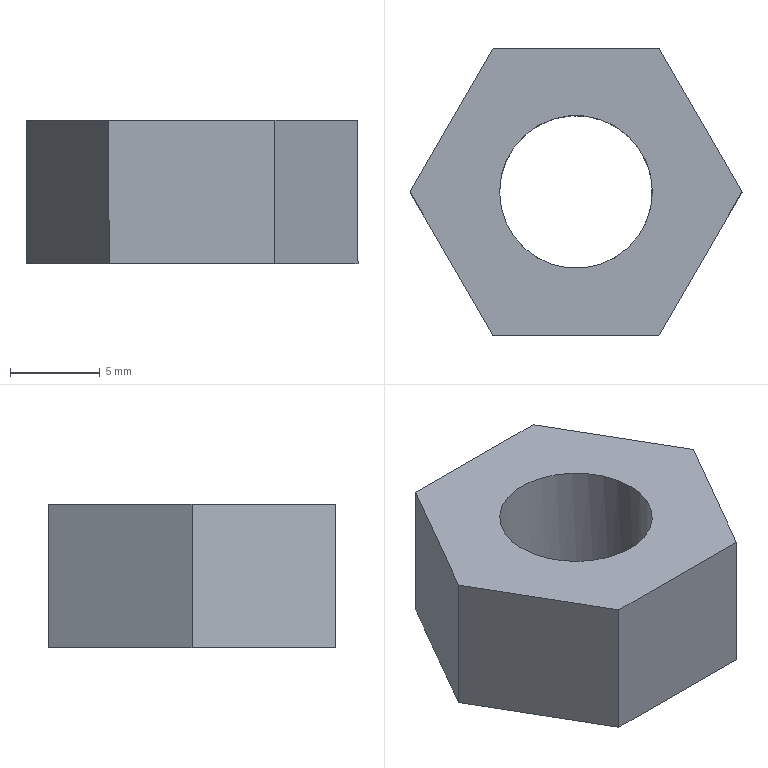Part | NX | 1 solid | 9 faces | box 18.475 x 16 x 8 mm | volume 1320 mm3 | plane 8 | cylinder 1 | commonest cylinder face diameters 8.5 x1
STEP:
#1=CARTESIAN_POINT('',(4.619,-8.,0.));
#2=VERTEX_POINT('',#1);
#3=CARTESIAN_POINT('',(9.238,0.,0.));
#4=VERTEX_POINT('',#3);
#5=CARTESIAN_POINT('',(4.619,-8.,0.));
#6=DIRECTION('',(0.5,0.866,0.));
#7=VECTOR('',#6,1000.);
#8=LINE('',#5,#7);
#9=EDGE_CURVE('',#2,#4,#8,.T.);
#10=ORIENTED_EDGE('',*,*,#9,.T.);
#11=CARTESIAN_POINT('',(9.238,0.,8.));
#12=VERTEX_POINT('',#11);
#13=CARTESIAN_POINT('',(9.238,0.,8.));
#14=DIRECTION('',(0.,0.,-1.));
#15=VECTOR('',#14,1000.);
#16=LINE('',#13,#15);
#17=EDGE_CURVE('',#12,#4,#16,.T.);
#18=ORIENTED_EDGE('',*,*,#17,.F.);
#19=CARTESIAN_POINT('',(4.619,-8.,8.));
#20=VERTEX_POINT('',#19);
#21=CARTESIAN_POINT('',(4.619,-8.,8.));
#22=DIRECTION('',(0.5,0.866,0.));
#23=VECTOR('',#22,1000.);
#24=LINE('',#21,#23);
#25=EDGE_CURVE('',#20,#12,#24,.T.);
#26=ORIENTED_EDGE('',*,*,#25,.F.);
#27=CARTESIAN_POINT('',(4.619,-8.,8.));
#28=DIRECTION('',(0.,0.,-1.));
#29=VECTOR('',#28,1000.);
#30=LINE('',#27,#29);
#31=EDGE_CURVE('',#20,#2,#30,.T.);
#32=ORIENTED_EDGE('',*,*,#31,.T.);
#33=EDGE_LOOP('',(#10,#18,#26,#32));
#34=FACE_BOUND('',#33,.T.);
#35=CARTESIAN_POINT('',(4.619,-8.,8.));
#36=DIRECTION('',(-0.866,0.5,0.));
#37=DIRECTION('',(-0.5,-0.866,0.));
#38=AXIS2_PLACEMENT_3D('',#35,#36,#37);
#39=PLANE('',#38);
#40=ADVANCED_FACE('',(#34),#39,.F.);
#41=CARTESIAN_POINT('',(4.619,8.,0.));
#42=VERTEX_POINT('',#41);
#43=CARTESIAN_POINT('',(9.238,0.,0.));
#44=DIRECTION('',(-0.5,0.866,0.));
#45=VECTOR('',#44,1000.);
#46=LINE('',#43,#45);
#47=EDGE_CURVE('',#4,#42,#46,.T.);
#48=ORIENTED_EDGE('',*,*,#47,.T.);
#49=CARTESIAN_POINT('',(4.619,8.,8.));
#50=VERTEX_POINT('',#49);
#51=CARTESIAN_POINT('',(4.619,8.,8.));
#52=DIRECTION('',(0.,0.,-1.));
#53=VECTOR('',#52,1000.);
#54=LINE('',#51,#53);
#55=EDGE_CURVE('',#50,#42,#54,.T.);
#56=ORIENTED_EDGE('',*,*,#55,.F.);
#57=CARTESIAN_POINT('',(9.238,0.,8.));
#58=DIRECTION('',(-0.5,0.866,0.));
#59=VECTOR('',#58,1000.);
#60=LINE('',#57,#59);
#61=EDGE_CURVE('',#12,#50,#60,.T.);
#62=ORIENTED_EDGE('',*,*,#61,.F.);
#63=ORIENTED_EDGE('',*,*,#17,.T.);
#64=EDGE_LOOP('',(#48,#56,#62,#63));
#65=FACE_BOUND('',#64,.T.);
#66=CARTESIAN_POINT('',(9.238,0.,8.));
#67=DIRECTION('',(-0.866,-0.5,0.));
#68=DIRECTION('',(0.5,-0.866,0.));
#69=AXIS2_PLACEMENT_3D('',#66,#67,#68);
#70=PLANE('',#69);
#71=ADVANCED_FACE('',(#65),#70,.F.);
#72=CARTESIAN_POINT('',(-4.619,8.,0.));
#73=VERTEX_POINT('',#72);
#74=CARTESIAN_POINT('',(4.619,8.,0.));
#75=DIRECTION('',(-1.,0.,0.));
#76=VECTOR('',#75,1000.);
#77=LINE('',#74,#76);
#78=EDGE_CURVE('',#42,#73,#77,.T.);
#79=ORIENTED_EDGE('',*,*,#78,.T.);
#80=CARTESIAN_POINT('',(-4.619,8.,8.));
#81=VERTEX_POINT('',#80);
#82=CARTESIAN_POINT('',(-4.619,8.,8.));
#83=DIRECTION('',(0.,0.,-1.));
#84=VECTOR('',#83,1000.);
#85=LINE('',#82,#84);
#86=EDGE_CURVE('',#81,#73,#85,.T.);
#87=ORIENTED_EDGE('',*,*,#86,.F.);
#88=CARTESIAN_POINT('',(4.619,8.,8.));
#89=DIRECTION('',(-1.,0.,0.));
#90=VECTOR('',#89,1000.);
#91=LINE('',#88,#90);
#92=EDGE_CURVE('',#50,#81,#91,.T.);
#93=ORIENTED_EDGE('',*,*,#92,.F.);
#94=ORIENTED_EDGE('',*,*,#55,.T.);
#95=EDGE_LOOP('',(#79,#87,#93,#94));
#96=FACE_BOUND('',#95,.T.);
#97=CARTESIAN_POINT('',(4.619,8.,8.));
#98=DIRECTION('',(0.,-1.,0.));
#99=DIRECTION('',(0.,0.,-1.));
#100=AXIS2_PLACEMENT_3D('',#97,#98,#99);
#101=PLANE('',#100);
#102=ADVANCED_FACE('',(#96),#101,.F.);
#103=CARTESIAN_POINT('',(-9.238,0.,0.));
#104=VERTEX_POINT('',#103);
#105=CARTESIAN_POINT('',(-4.619,8.,0.));
#106=DIRECTION('',(-0.5,-0.866,0.));
#107=VECTOR('',#106,1000.);
#108=LINE('',#105,#107);
#109=EDGE_CURVE('',#73,#104,#108,.T.);
#110=ORIENTED_EDGE('',*,*,#109,.T.);
#111=CARTESIAN_POINT('',(-9.238,0.,8.));
#112=VERTEX_POINT('',#111);
#113=CARTESIAN_POINT('',(-9.238,0.,8.));
#114=DIRECTION('',(0.,0.,-1.));
#115=VECTOR('',#114,1000.);
#116=LINE('',#113,#115);
#117=EDGE_CURVE('',#112,#104,#116,.T.);
#118=ORIENTED_EDGE('',*,*,#117,.F.);
#119=CARTESIAN_POINT('',(-4.619,8.,8.));
#120=DIRECTION('',(-0.5,-0.866,0.));
#121=VECTOR('',#120,1000.);
#122=LINE('',#119,#121);
#123=EDGE_CURVE('',#81,#112,#122,.T.);
#124=ORIENTED_EDGE('',*,*,#123,.F.);
#125=ORIENTED_EDGE('',*,*,#86,.T.);
#126=EDGE_LOOP('',(#110,#118,#124,#125));
#127=FACE_BOUND('',#126,.T.);
#128=CARTESIAN_POINT('',(-4.619,8.,8.));
#129=DIRECTION('',(0.866,-0.5,0.));
#130=DIRECTION('',(0.5,0.866,0.));
#131=AXIS2_PLACEMENT_3D('',#128,#129,#130);
#132=PLANE('',#131);
#133=ADVANCED_FACE('',(#127),#132,.F.);
#134=CARTESIAN_POINT('',(-4.619,-8.,0.));
#135=VERTEX_POINT('',#134);
#136=CARTESIAN_POINT('',(-9.238,0.,0.));
#137=DIRECTION('',(0.5,-0.866,0.));
#138=VECTOR('',#137,1000.);
#139=LINE('',#136,#138);
#140=EDGE_CURVE('',#104,#135,#139,.T.);
#141=ORIENTED_EDGE('',*,*,#140,.T.);
#142=CARTESIAN_POINT('',(-4.619,-8.,8.));
#143=VERTEX_POINT('',#142);
#144=CARTESIAN_POINT('',(-4.619,-8.,8.));
#145=DIRECTION('',(0.,0.,-1.));
#146=VECTOR('',#145,1000.);
#147=LINE('',#144,#146);
#148=EDGE_CURVE('',#143,#135,#147,.T.);
#149=ORIENTED_EDGE('',*,*,#148,.F.);
#150=CARTESIAN_POINT('',(-9.238,0.,8.));
#151=DIRECTION('',(0.5,-0.866,0.));
#152=VECTOR('',#151,1000.);
#153=LINE('',#150,#152);
#154=EDGE_CURVE('',#112,#143,#153,.T.);
#155=ORIENTED_EDGE('',*,*,#154,.F.);
#156=ORIENTED_EDGE('',*,*,#117,.T.);
#157=EDGE_LOOP('',(#141,#149,#155,#156));
#158=FACE_BOUND('',#157,.T.);
#159=CARTESIAN_POINT('',(-9.238,0.,8.));
#160=DIRECTION('',(0.866,0.5,0.));
#161=DIRECTION('',(-0.5,0.866,0.));
#162=AXIS2_PLACEMENT_3D('',#159,#160,#161);
#163=PLANE('',#162);
#164=ADVANCED_FACE('',(#158),#163,.F.);
#165=CARTESIAN_POINT('',(-4.619,-8.,0.));
#166=DIRECTION('',(1.,0.,0.));
#167=VECTOR('',#166,1000.);
#168=LINE('',#165,#167);
#169=EDGE_CURVE('',#135,#2,#168,.T.);
#170=ORIENTED_EDGE('',*,*,#169,.T.);
#171=ORIENTED_EDGE('',*,*,#31,.F.);
#172=CARTESIAN_POINT('',(-4.619,-8.,8.));
#173=DIRECTION('',(1.,0.,0.));
#174=VECTOR('',#173,1000.);
#175=LINE('',#172,#174);
#176=EDGE_CURVE('',#143,#20,#175,.T.);
#177=ORIENTED_EDGE('',*,*,#176,.F.);
#178=ORIENTED_EDGE('',*,*,#148,.T.);
#179=EDGE_LOOP('',(#170,#171,#177,#178));
#180=FACE_BOUND('',#179,.T.);
#181=CARTESIAN_POINT('',(-4.619,-8.,8.));
#182=DIRECTION('',(0.,1.,0.));
#183=DIRECTION('',(-1.,0.,0.));
#184=AXIS2_PLACEMENT_3D('',#181,#182,#183);
#185=PLANE('',#184);
#186=ADVANCED_FACE('',(#180),#185,.F.);
#187=CARTESIAN_POINT('',(4.25,0.,8.));
#188=VERTEX_POINT('',#187);
#189=CARTESIAN_POINT('',(0.,0.,8.));
#190=DIRECTION('',(0.,0.,1.));
#191=DIRECTION('',(1.,0.,0.));
#192=AXIS2_PLACEMENT_3D('',#189,#190,#191);
#193=CIRCLE('',#192,4.25);
#194=EDGE_CURVE('',#188,#188,#193,.T.);
#195=ORIENTED_EDGE('',*,*,#194,.F.);
#196=EDGE_LOOP('',(#195));
#197=FACE_BOUND('',#196,.T.);
#198=ORIENTED_EDGE('',*,*,#25,.T.);
#199=ORIENTED_EDGE('',*,*,#61,.T.);
#200=ORIENTED_EDGE('',*,*,#92,.T.);
#201=ORIENTED_EDGE('',*,*,#123,.T.);
#202=ORIENTED_EDGE('',*,*,#154,.T.);
#203=ORIENTED_EDGE('',*,*,#176,.T.);
#204=EDGE_LOOP('',(#198,#199,#200,#201,#202,#203));
#205=FACE_BOUND('',#204,.T.);
#206=CARTESIAN_POINT('',(0.,0.,8.));
#207=DIRECTION('',(0.,0.,1.));
#208=DIRECTION('',(1.,0.,0.));
#209=AXIS2_PLACEMENT_3D('',#206,#207,#208);
#210=PLANE('',#209);
#211=ADVANCED_FACE('',(#197,#205),#210,.T.);
#212=CARTESIAN_POINT('',(-4.25,0.,0.));
#213=VERTEX_POINT('',#212);
#214=CARTESIAN_POINT('',(0.,0.,0.));
#215=DIRECTION('',(0.,0.,-1.));
#216=DIRECTION('',(-1.,0.,0.));
#217=AXIS2_PLACEMENT_3D('',#214,#215,#216);
#218=CIRCLE('',#217,4.25);
#219=EDGE_CURVE('',#213,#213,#218,.T.);
#220=ORIENTED_EDGE('',*,*,#219,.F.);
#221=EDGE_LOOP('',(#220));
#222=FACE_BOUND('',#221,.T.);
#223=ORIENTED_EDGE('',*,*,#9,.F.);
#224=ORIENTED_EDGE('',*,*,#169,.F.);
#225=ORIENTED_EDGE('',*,*,#140,.F.);
#226=ORIENTED_EDGE('',*,*,#109,.F.);
#227=ORIENTED_EDGE('',*,*,#78,.F.);
#228=ORIENTED_EDGE('',*,*,#47,.F.);
#229=EDGE_LOOP('',(#223,#224,#225,#226,#227,#228));
#230=FACE_BOUND('',#229,.T.);
#231=CARTESIAN_POINT('',(0.,0.,0.));
#232=DIRECTION('',(0.,0.,1.));
#233=DIRECTION('',(1.,0.,0.));
#234=AXIS2_PLACEMENT_3D('',#231,#232,#233);
#235=PLANE('',#234);
#236=ADVANCED_FACE('',(#222,#230),#235,.F.);
#237=ORIENTED_EDGE('',*,*,#194,.T.);
#238=EDGE_LOOP('',(#237));
#239=FACE_BOUND('',#238,.T.);
#240=ORIENTED_EDGE('',*,*,#219,.T.);
#241=EDGE_LOOP('',(#240));
#242=FACE_BOUND('',#241,.T.);
#243=CARTESIAN_POINT('',(0.,0.,0.));
#244=DIRECTION('',(0.,0.,-1.));
#245=DIRECTION('',(-1.,0.,0.));
#246=AXIS2_PLACEMENT_3D('',#243,#244,#245);
#247=CYLINDRICAL_SURFACE('',#246,4.25);
#248=ADVANCED_FACE('',(#239,#242),#247,.F.);
#249=CLOSED_SHELL('',(#40,#71,#102,#133,#164,#186,#211,#236,#248));
#250=MANIFOLD_SOLID_BREP('',#249);
#251=(LENGTH_UNIT()NAMED_UNIT(*)SI_UNIT(.MILLI.,.METRE.));
#252=UNCERTAINTY_MEASURE_WITH_UNIT(LENGTH_MEASURE(0.00001),#251,'','');
#253=(NAMED_UNIT(*)PLANE_ANGLE_UNIT()SI_UNIT($,.RADIAN.));
#254=(NAMED_UNIT(*)SI_UNIT($,.STERADIAN.)SOLID_ANGLE_UNIT());
#255=(GEOMETRIC_REPRESENTATION_CONTEXT(3)GLOBAL_UNCERTAINTY_ASSIGNED_CONTEXT((#252))GLOBAL_UNIT_ASSIGNED_CONTEXT((#251,#253,#254))REPRESENTATION_CONTEXT('',''));
#256=ADVANCED_BREP_SHAPE_REPRESENTATION('',(#250),#255);